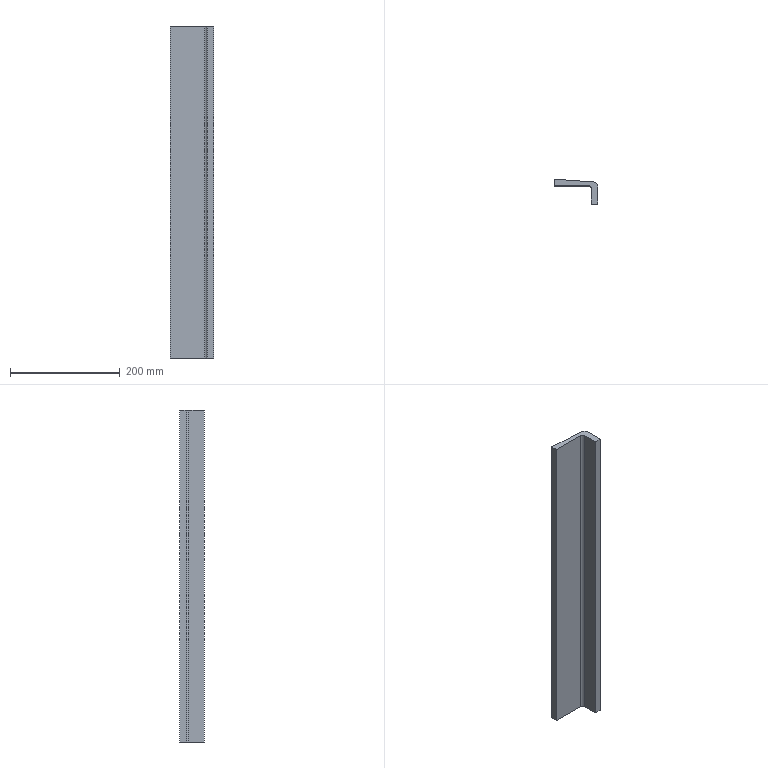Part | STEP file | daozhiban | 1 solid | 10 faces | box 80 x 45.5 x 606 mm | volume 689617 mm3 | plane 8 | cylinder 2 | commonest cylinder face diameters 10 x1 20 x1
STEP:
#1=CARTESIAN_POINT('',(0.,0.,0.));
#2=DIRECTION('',(0.,0.,1.));
#3=DIRECTION('',(1.,0.,0.));
#4=AXIS2_PLACEMENT_3D('',#1,#2,#3);
#5=CARTESIAN_POINT('',(36.453,-0.6319,-303.));
#6=VERTEX_POINT('',#5);
#7=CARTESIAN_POINT('',(29.053,9.024,-303.));
#8=VERTEX_POINT('',#7);
#9=CARTESIAN_POINT('',(26.453,-0.6319,-303.));
#10=DIRECTION('',(0.,0.,1.));
#11=DIRECTION('',(-1.,0.,0.));
#12=AXIS2_PLACEMENT_3D('',#9,#10,#11);
#13=CIRCLE('',#12,10.);
#14=CARTESIAN_POINT('',(26.453,-0.6319,303.));
#15=DIRECTION('',(0.,0.,-1.));
#16=DIRECTION('',(-1.,0.,0.));
#17=AXIS2_PLACEMENT_3D('',#14,#15,#16);
#18=CYLINDRICAL_SURFACE('',#17,10.);
#19=CARTESIAN_POINT('',(6.283,606.));
#20=DIRECTION('',(-1.,0.));
#21=VECTOR('',#20,1.);
#22=LINE('',#19,#21);
#23=(GEOMETRIC_REPRESENTATION_CONTEXT(2)PARAMETRIC_REPRESENTATION_CONTEXT()REPRESENTATION_CONTEXT('',''));
#24=DEFINITIONAL_REPRESENTATION('',(#22),#23);
#25=PCURVE('',#18,#24);
#26=CARTESIAN_POINT('',(26.453,-0.6319,-303.));
#27=DIRECTION('',(0.,0.,-1.));
#28=DIRECTION('',(-1.,0.,0.));
#29=AXIS2_PLACEMENT_3D('',#26,#27,#28);
#30=PLANE('',#29);
#31=CARTESIAN_POINT('',(10.,0.));
#32=CARTESIAN_POINT('',(10.,-17.321));
#33=CARTESIAN_POINT('',(-5.,-8.66));
#34=CARTESIAN_POINT('',(-20.,0.));
#35=CARTESIAN_POINT('',(-5.,8.66));
#36=CARTESIAN_POINT('',(10.,17.321));
#37=CARTESIAN_POINT('',(10.,0.));
#38=(BOUNDED_CURVE()B_SPLINE_CURVE(2,(#31,#32,#33,#34,#35,#36,#37),.UNSPECIFIED.,.T.,.F.)B_SPLINE_CURVE_WITH_KNOTS((1,2,2,2,2,1),(-2.094,0.,2.094,4.189,6.283,8.378),.UNSPECIFIED.)CURVE()GEOMETRIC_REPRESENTATION_ITEM()RATIONAL_B_SPLINE_CURVE((1.,0.5,1.,0.5,1.,0.5,1.))REPRESENTATION_ITEM(''));
#39=(GEOMETRIC_REPRESENTATION_CONTEXT(2)PARAMETRIC_REPRESENTATION_CONTEXT()REPRESENTATION_CONTEXT('',''));
#40=DEFINITIONAL_REPRESENTATION('',(#38),#39);
#41=PCURVE('',#30,#40);
#42=SURFACE_CURVE('',#13,(#25,#41),.PCURVE_S1.);
#43=EDGE_CURVE('',#6,#8,#42,.T.);
#44=ORIENTED_EDGE('',*,*,#43,.T.);
#45=CARTESIAN_POINT('',(29.053,9.024,303.));
#46=VERTEX_POINT('',#45);
#47=CARTESIAN_POINT('',(29.053,9.024,303.));
#48=DIRECTION('',(0.,0.,-1.));
#49=VECTOR('',#48,1.);
#50=LINE('',#47,#49);
#51=CARTESIAN_POINT('',(1.834,0.));
#52=DIRECTION('',(0.,1.));
#53=VECTOR('',#52,1.);
#54=LINE('',#51,#53);
#55=(GEOMETRIC_REPRESENTATION_CONTEXT(2)PARAMETRIC_REPRESENTATION_CONTEXT()REPRESENTATION_CONTEXT('',''));
#56=DEFINITIONAL_REPRESENTATION('',(#54),#55);
#57=PCURVE('',#18,#56);
#58=CARTESIAN_POINT('',(-43.547,13.847,303.));
#59=DIRECTION('',(-0.06629,-0.9978,0.));
#60=DIRECTION('',(0.9978,-0.06629,0.));
#61=AXIS2_PLACEMENT_3D('',#58,#59,#60);
#62=PLANE('',#61);
#63=CARTESIAN_POINT('',(72.76,0.));
#64=DIRECTION('',(0.,-1.));
#65=VECTOR('',#64,1.);
#66=LINE('',#63,#65);
#67=(GEOMETRIC_REPRESENTATION_CONTEXT(2)PARAMETRIC_REPRESENTATION_CONTEXT()REPRESENTATION_CONTEXT('',''));
#68=DEFINITIONAL_REPRESENTATION('',(#66),#67);
#69=PCURVE('',#62,#68);
#70=SURFACE_CURVE('',#50,(#57,#69),.PCURVE_S1.);
#71=EDGE_CURVE('',#46,#8,#70,.T.);
#72=ORIENTED_EDGE('',*,*,#71,.F.);
#73=CARTESIAN_POINT('',(36.453,-0.6319,303.));
#74=VERTEX_POINT('',#73);
#75=CARTESIAN_POINT('',(26.453,-0.6319,303.));
#76=DIRECTION('',(0.,0.,1.));
#77=DIRECTION('',(-1.,0.,0.));
#78=AXIS2_PLACEMENT_3D('',#75,#76,#77);
#79=CIRCLE('',#78,10.);
#80=CARTESIAN_POINT('',(6.283,0.));
#81=DIRECTION('',(-1.,0.));
#82=VECTOR('',#81,1.);
#83=LINE('',#80,#82);
#84=(GEOMETRIC_REPRESENTATION_CONTEXT(2)PARAMETRIC_REPRESENTATION_CONTEXT()REPRESENTATION_CONTEXT('',''));
#85=DEFINITIONAL_REPRESENTATION('',(#83),#84);
#86=PCURVE('',#18,#85);
#87=CARTESIAN_POINT('',(26.453,-0.6319,303.));
#88=DIRECTION('',(0.,0.,-1.));
#89=DIRECTION('',(-1.,0.,0.));
#90=AXIS2_PLACEMENT_3D('',#87,#88,#89);
#91=PLANE('',#90);
#92=CARTESIAN_POINT('',(10.,0.));
#93=CARTESIAN_POINT('',(10.,-17.321));
#94=CARTESIAN_POINT('',(-5.,-8.66));
#95=CARTESIAN_POINT('',(-20.,0.));
#96=CARTESIAN_POINT('',(-5.,8.66));
#97=CARTESIAN_POINT('',(10.,17.321));
#98=CARTESIAN_POINT('',(10.,0.));
#99=(BOUNDED_CURVE()B_SPLINE_CURVE(2,(#92,#93,#94,#95,#96,#97,#98),.UNSPECIFIED.,.T.,.F.)B_SPLINE_CURVE_WITH_KNOTS((1,2,2,2,2,1),(-2.094,0.,2.094,4.189,6.283,8.378),.UNSPECIFIED.)CURVE()GEOMETRIC_REPRESENTATION_ITEM()RATIONAL_B_SPLINE_CURVE((1.,0.5,1.,0.5,1.,0.5,1.))REPRESENTATION_ITEM(''));
#100=(GEOMETRIC_REPRESENTATION_CONTEXT(2)PARAMETRIC_REPRESENTATION_CONTEXT()REPRESENTATION_CONTEXT('',''));
#101=DEFINITIONAL_REPRESENTATION('',(#99),#100);
#102=PCURVE('',#91,#101);
#103=SURFACE_CURVE('',#79,(#86,#102),.PCURVE_S1.);
#104=EDGE_CURVE('',#74,#46,#103,.T.);
#105=ORIENTED_EDGE('',*,*,#104,.F.);
#106=CARTESIAN_POINT('',(36.453,-0.6319,303.));
#107=DIRECTION('',(0.,0.,-1.));
#108=VECTOR('',#107,1.);
#109=LINE('',#106,#108);
#110=CARTESIAN_POINT('',(3.142,0.));
#111=DIRECTION('',(0.,1.));
#112=VECTOR('',#111,1.);
#113=LINE('',#110,#112);
#114=(GEOMETRIC_REPRESENTATION_CONTEXT(2)PARAMETRIC_REPRESENTATION_CONTEXT()REPRESENTATION_CONTEXT('',''));
#115=DEFINITIONAL_REPRESENTATION('',(#113),#114);
#116=PCURVE('',#18,#115);
#117=CARTESIAN_POINT('',(36.453,-0.6319,303.));
#118=DIRECTION('',(-1.,0.,0.));
#119=DIRECTION('',(0.,-1.,0.));
#120=AXIS2_PLACEMENT_3D('',#117,#118,#119);
#121=PLANE('',#120);
#122=CARTESIAN_POINT('',(0.,0.));
#123=DIRECTION('',(0.,-1.));
#124=VECTOR('',#123,1.);
#125=LINE('',#122,#124);
#126=(GEOMETRIC_REPRESENTATION_CONTEXT(2)PARAMETRIC_REPRESENTATION_CONTEXT()REPRESENTATION_CONTEXT('',''));
#127=DEFINITIONAL_REPRESENTATION('',(#125),#126);
#128=PCURVE('',#121,#127);
#129=SURFACE_CURVE('',#109,(#116,#128),.PCURVE_S1.);
#130=EDGE_CURVE('',#74,#6,#129,.T.);
#131=ORIENTED_EDGE('',*,*,#130,.T.);
#132=EDGE_LOOP('',(#44,#72,#105,#131));
#133=FACE_BOUND('',#132,.T.);
#134=ADVANCED_FACE('',(#133),#18,.T.);
#135=CARTESIAN_POINT('',(-43.547,13.847,-303.));
#136=VERTEX_POINT('',#135);
#137=CARTESIAN_POINT('',(-43.547,13.847,-303.));
#138=DIRECTION('',(-0.9978,0.06629,0.));
#139=VECTOR('',#138,1.);
#140=LINE('',#137,#139);
#141=CARTESIAN_POINT('',(0.,-606.));
#142=DIRECTION('',(-1.,0.));
#143=VECTOR('',#142,1.);
#144=LINE('',#141,#143);
#145=(GEOMETRIC_REPRESENTATION_CONTEXT(2)PARAMETRIC_REPRESENTATION_CONTEXT()REPRESENTATION_CONTEXT('',''));
#146=DEFINITIONAL_REPRESENTATION('',(#144),#145);
#147=PCURVE('',#62,#146);
#148=CARTESIAN_POINT('',(70.,14.479));
#149=DIRECTION('',(0.9978,0.06629));
#150=VECTOR('',#149,1.);
#151=LINE('',#148,#150);
#152=(GEOMETRIC_REPRESENTATION_CONTEXT(2)PARAMETRIC_REPRESENTATION_CONTEXT()REPRESENTATION_CONTEXT('',''));
#153=DEFINITIONAL_REPRESENTATION('',(#151),#152);
#154=PCURVE('',#30,#153);
#155=SURFACE_CURVE('',#140,(#147,#154),.PCURVE_S1.);
#156=EDGE_CURVE('',#8,#136,#155,.T.);
#157=ORIENTED_EDGE('',*,*,#156,.T.);
#158=CARTESIAN_POINT('',(-43.547,13.847,303.));
#159=VERTEX_POINT('',#158);
#160=CARTESIAN_POINT('',(-43.547,13.847,303.));
#161=DIRECTION('',(0.,0.,-1.));
#162=VECTOR('',#161,1.);
#163=LINE('',#160,#162);
#164=CARTESIAN_POINT('',(0.,0.));
#165=DIRECTION('',(0.,-1.));
#166=VECTOR('',#165,1.);
#167=LINE('',#164,#166);
#168=(GEOMETRIC_REPRESENTATION_CONTEXT(2)PARAMETRIC_REPRESENTATION_CONTEXT()REPRESENTATION_CONTEXT('',''));
#169=DEFINITIONAL_REPRESENTATION('',(#167),#168);
#170=PCURVE('',#62,#169);
#171=CARTESIAN_POINT('',(-43.547,13.847,303.));
#172=DIRECTION('',(1.,0.,0.));
#173=DIRECTION('',(0.,0.,-1.));
#174=AXIS2_PLACEMENT_3D('',#171,#172,#173);
#175=PLANE('',#174);
#176=CARTESIAN_POINT('',(0.,0.));
#177=DIRECTION('',(1.,0.));
#178=VECTOR('',#177,1.);
#179=LINE('',#176,#178);
#180=(GEOMETRIC_REPRESENTATION_CONTEXT(2)PARAMETRIC_REPRESENTATION_CONTEXT()REPRESENTATION_CONTEXT('',''));
#181=DEFINITIONAL_REPRESENTATION('',(#179),#180);
#182=PCURVE('',#175,#181);
#183=SURFACE_CURVE('',#163,(#170,#182),.PCURVE_S1.);
#184=EDGE_CURVE('',#159,#136,#183,.T.);
#185=ORIENTED_EDGE('',*,*,#184,.F.);
#186=CARTESIAN_POINT('',(-43.547,13.847,303.));
#187=DIRECTION('',(-0.9978,0.06629,0.));
#188=VECTOR('',#187,1.);
#189=LINE('',#186,#188);
#190=CARTESIAN_POINT('',(0.,0.));
#191=DIRECTION('',(-1.,0.));
#192=VECTOR('',#191,1.);
#193=LINE('',#190,#192);
#194=(GEOMETRIC_REPRESENTATION_CONTEXT(2)PARAMETRIC_REPRESENTATION_CONTEXT()REPRESENTATION_CONTEXT('',''));
#195=DEFINITIONAL_REPRESENTATION('',(#193),#194);
#196=PCURVE('',#62,#195);
#197=CARTESIAN_POINT('',(70.,14.479));
#198=DIRECTION('',(0.9978,0.06629));
#199=VECTOR('',#198,1.);
#200=LINE('',#197,#199);
#201=(GEOMETRIC_REPRESENTATION_CONTEXT(2)PARAMETRIC_REPRESENTATION_CONTEXT()REPRESENTATION_CONTEXT('',''));
#202=DEFINITIONAL_REPRESENTATION('',(#200),#201);
#203=PCURVE('',#91,#202);
#204=SURFACE_CURVE('',#189,(#196,#203),.PCURVE_S1.);
#205=EDGE_CURVE('',#46,#159,#204,.T.);
#206=ORIENTED_EDGE('',*,*,#205,.F.);
#207=ORIENTED_EDGE('',*,*,#71,.T.);
#208=EDGE_LOOP('',(#157,#185,#206,#207));
#209=FACE_BOUND('',#208,.T.);
#210=ADVANCED_FACE('',(#209),#62,.F.);
#211=CARTESIAN_POINT('',(-43.547,1.847,-303.));
#212=VERTEX_POINT('',#211);
#213=CARTESIAN_POINT('',(-43.547,13.847,-303.));
#214=DIRECTION('',(0.,-1.,0.));
#215=VECTOR('',#214,1.);
#216=LINE('',#213,#215);
#217=CARTESIAN_POINT('',(606.,0.));
#218=DIRECTION('',(0.,-1.));
#219=VECTOR('',#218,1.);
#220=LINE('',#217,#219);
#221=(GEOMETRIC_REPRESENTATION_CONTEXT(2)PARAMETRIC_REPRESENTATION_CONTEXT()REPRESENTATION_CONTEXT('',''));
#222=DEFINITIONAL_REPRESENTATION('',(#220),#221);
#223=PCURVE('',#175,#222);
#224=CARTESIAN_POINT('',(70.,14.479));
#225=DIRECTION('',(0.,-1.));
#226=VECTOR('',#225,1.);
#227=LINE('',#224,#226);
#228=(GEOMETRIC_REPRESENTATION_CONTEXT(2)PARAMETRIC_REPRESENTATION_CONTEXT()REPRESENTATION_CONTEXT('',''));
#229=DEFINITIONAL_REPRESENTATION('',(#227),#228);
#230=PCURVE('',#30,#229);
#231=SURFACE_CURVE('',#216,(#223,#230),.PCURVE_S1.);
#232=EDGE_CURVE('',#136,#212,#231,.T.);
#233=ORIENTED_EDGE('',*,*,#232,.T.);
#234=CARTESIAN_POINT('',(-43.547,1.847,303.));
#235=VERTEX_POINT('',#234);
#236=CARTESIAN_POINT('',(-43.547,1.847,303.));
#237=DIRECTION('',(0.,0.,-1.));
#238=VECTOR('',#237,1.);
#239=LINE('',#236,#238);
#240=CARTESIAN_POINT('',(0.,-12.));
#241=DIRECTION('',(1.,0.));
#242=VECTOR('',#241,1.);
#243=LINE('',#240,#242);
#244=(GEOMETRIC_REPRESENTATION_CONTEXT(2)PARAMETRIC_REPRESENTATION_CONTEXT()REPRESENTATION_CONTEXT('',''));
#245=DEFINITIONAL_REPRESENTATION('',(#243),#244);
#246=PCURVE('',#175,#245);
#247=CARTESIAN_POINT('',(-43.547,1.847,303.));
#248=DIRECTION('',(0.,1.,0.));
#249=DIRECTION('',(0.,0.,1.));
#250=AXIS2_PLACEMENT_3D('',#247,#248,#249);
#251=PLANE('',#250);
#252=CARTESIAN_POINT('',(0.,0.));
#253=DIRECTION('',(-1.,0.));
#254=VECTOR('',#253,1.);
#255=LINE('',#252,#254);
#256=(GEOMETRIC_REPRESENTATION_CONTEXT(2)PARAMETRIC_REPRESENTATION_CONTEXT()REPRESENTATION_CONTEXT('',''));
#257=DEFINITIONAL_REPRESENTATION('',(#255),#256);
#258=PCURVE('',#251,#257);
#259=SURFACE_CURVE('',#239,(#246,#258),.PCURVE_S1.);
#260=EDGE_CURVE('',#235,#212,#259,.T.);
#261=ORIENTED_EDGE('',*,*,#260,.F.);
#262=CARTESIAN_POINT('',(-43.547,13.847,303.));
#263=DIRECTION('',(0.,-1.,0.));
#264=VECTOR('',#263,1.);
#265=LINE('',#262,#264);
#266=CARTESIAN_POINT('',(0.,0.));
#267=DIRECTION('',(0.,-1.));
#268=VECTOR('',#267,1.);
#269=LINE('',#266,#268);
#270=(GEOMETRIC_REPRESENTATION_CONTEXT(2)PARAMETRIC_REPRESENTATION_CONTEXT()REPRESENTATION_CONTEXT('',''));
#271=DEFINITIONAL_REPRESENTATION('',(#269),#270);
#272=PCURVE('',#175,#271);
#273=CARTESIAN_POINT('',(70.,14.479));
#274=DIRECTION('',(0.,-1.));
#275=VECTOR('',#274,1.);
#276=LINE('',#273,#275);
#277=(GEOMETRIC_REPRESENTATION_CONTEXT(2)PARAMETRIC_REPRESENTATION_CONTEXT()REPRESENTATION_CONTEXT('',''));
#278=DEFINITIONAL_REPRESENTATION('',(#276),#277);
#279=PCURVE('',#91,#278);
#280=SURFACE_CURVE('',#265,(#272,#279),.PCURVE_S1.);
#281=EDGE_CURVE('',#159,#235,#280,.T.);
#282=ORIENTED_EDGE('',*,*,#281,.F.);
#283=ORIENTED_EDGE('',*,*,#184,.T.);
#284=EDGE_LOOP('',(#233,#261,#282,#283));
#285=FACE_BOUND('',#284,.T.);
#286=ADVANCED_FACE('',(#285),#175,.F.);
#287=CARTESIAN_POINT('',(19.453,1.847,-303.));
#288=VERTEX_POINT('',#287);
#289=CARTESIAN_POINT('',(-43.547,1.847,-303.));
#290=DIRECTION('',(1.,0.,0.));
#291=VECTOR('',#290,1.);
#292=LINE('',#289,#291);
#293=CARTESIAN_POINT('',(-606.,0.));
#294=DIRECTION('',(0.,1.));
#295=VECTOR('',#294,1.);
#296=LINE('',#293,#295);
#297=(GEOMETRIC_REPRESENTATION_CONTEXT(2)PARAMETRIC_REPRESENTATION_CONTEXT()REPRESENTATION_CONTEXT('',''));
#298=DEFINITIONAL_REPRESENTATION('',(#296),#297);
#299=PCURVE('',#251,#298);
#300=CARTESIAN_POINT('',(70.,2.479));
#301=DIRECTION('',(-1.,0.));
#302=VECTOR('',#301,1.);
#303=LINE('',#300,#302);
#304=(GEOMETRIC_REPRESENTATION_CONTEXT(2)PARAMETRIC_REPRESENTATION_CONTEXT()REPRESENTATION_CONTEXT('',''));
#305=DEFINITIONAL_REPRESENTATION('',(#303),#304);
#306=PCURVE('',#30,#305);
#307=SURFACE_CURVE('',#292,(#299,#306),.PCURVE_S1.);
#308=EDGE_CURVE('',#212,#288,#307,.T.);
#309=ORIENTED_EDGE('',*,*,#308,.T.);
#310=CARTESIAN_POINT('',(19.453,1.847,303.));
#311=VERTEX_POINT('',#310);
#312=CARTESIAN_POINT('',(19.453,1.847,303.));
#313=DIRECTION('',(0.,0.,1.));
#314=VECTOR('',#313,1.);
#315=LINE('',#312,#314);
#316=CARTESIAN_POINT('',(0.,63.));
#317=DIRECTION('',(1.,0.));
#318=VECTOR('',#317,1.);
#319=LINE('',#316,#318);
#320=(GEOMETRIC_REPRESENTATION_CONTEXT(2)PARAMETRIC_REPRESENTATION_CONTEXT()REPRESENTATION_CONTEXT('',''));
#321=DEFINITIONAL_REPRESENTATION('',(#319),#320);
#322=PCURVE('',#251,#321);
#323=CARTESIAN_POINT('',(19.453,-3.153,303.));
#324=DIRECTION('',(0.,0.,1.));
#325=DIRECTION('',(1.,0.,0.));
#326=AXIS2_PLACEMENT_3D('',#323,#324,#325);
#327=CYLINDRICAL_SURFACE('',#326,5.);
#328=CARTESIAN_POINT('',(1.571,0.));
#329=DIRECTION('',(0.,1.));
#330=VECTOR('',#329,1.);
#331=LINE('',#328,#330);
#332=(GEOMETRIC_REPRESENTATION_CONTEXT(2)PARAMETRIC_REPRESENTATION_CONTEXT()REPRESENTATION_CONTEXT('',''));
#333=DEFINITIONAL_REPRESENTATION('',(#331),#332);
#334=PCURVE('',#327,#333);
#335=SURFACE_CURVE('',#315,(#322,#334),.PCURVE_S1.);
#336=EDGE_CURVE('',#288,#311,#335,.T.);
#337=ORIENTED_EDGE('',*,*,#336,.T.);
#338=CARTESIAN_POINT('',(-43.547,1.847,303.));
#339=DIRECTION('',(1.,0.,0.));
#340=VECTOR('',#339,1.);
#341=LINE('',#338,#340);
#342=CARTESIAN_POINT('',(0.,0.));
#343=DIRECTION('',(0.,1.));
#344=VECTOR('',#343,1.);
#345=LINE('',#342,#344);
#346=(GEOMETRIC_REPRESENTATION_CONTEXT(2)PARAMETRIC_REPRESENTATION_CONTEXT()REPRESENTATION_CONTEXT('',''));
#347=DEFINITIONAL_REPRESENTATION('',(#345),#346);
#348=PCURVE('',#251,#347);
#349=CARTESIAN_POINT('',(70.,2.479));
#350=DIRECTION('',(-1.,0.));
#351=VECTOR('',#350,1.);
#352=LINE('',#349,#351);
#353=(GEOMETRIC_REPRESENTATION_CONTEXT(2)PARAMETRIC_REPRESENTATION_CONTEXT()REPRESENTATION_CONTEXT('',''));
#354=DEFINITIONAL_REPRESENTATION('',(#352),#353);
#355=PCURVE('',#91,#354);
#356=SURFACE_CURVE('',#341,(#348,#355),.PCURVE_S1.);
#357=EDGE_CURVE('',#235,#311,#356,.T.);
#358=ORIENTED_EDGE('',*,*,#357,.F.);
#359=ORIENTED_EDGE('',*,*,#260,.T.);
#360=EDGE_LOOP('',(#309,#337,#358,#359));
#361=FACE_BOUND('',#360,.T.);
#362=ADVANCED_FACE('',(#361),#251,.F.);
#363=CARTESIAN_POINT('',(24.453,-3.153,303.));
#364=VERTEX_POINT('',#363);
#365=CARTESIAN_POINT('',(24.453,-31.653,303.));
#366=VERTEX_POINT('',#365);
#367=CARTESIAN_POINT('',(24.453,1.847,303.));
#368=DIRECTION('',(0.,-1.,0.));
#369=VECTOR('',#368,1.);
#370=LINE('',#367,#369);
#371=CARTESIAN_POINT('',(24.453,1.847,303.));
#372=DIRECTION('',(1.,0.,0.));
#373=DIRECTION('',(0.,1.,0.));
#374=AXIS2_PLACEMENT_3D('',#371,#372,#373);
#375=PLANE('',#374);
#376=CARTESIAN_POINT('',(0.,0.));
#377=DIRECTION('',(-1.,0.));
#378=VECTOR('',#377,1.);
#379=LINE('',#376,#378);
#380=(GEOMETRIC_REPRESENTATION_CONTEXT(2)PARAMETRIC_REPRESENTATION_CONTEXT()REPRESENTATION_CONTEXT('',''));
#381=DEFINITIONAL_REPRESENTATION('',(#379),#380);
#382=PCURVE('',#375,#381);
#383=CARTESIAN_POINT('',(2.,2.479));
#384=DIRECTION('',(0.,-1.));
#385=VECTOR('',#384,1.);
#386=LINE('',#383,#385);
#387=(GEOMETRIC_REPRESENTATION_CONTEXT(2)PARAMETRIC_REPRESENTATION_CONTEXT()REPRESENTATION_CONTEXT('',''));
#388=DEFINITIONAL_REPRESENTATION('',(#386),#387);
#389=PCURVE('',#91,#388);
#390=SURFACE_CURVE('',#370,(#382,#389),.PCURVE_S1.);
#391=EDGE_CURVE('',#364,#366,#390,.T.);
#392=ORIENTED_EDGE('',*,*,#391,.F.);
#393=CARTESIAN_POINT('',(24.453,-3.153,-303.));
#394=VERTEX_POINT('',#393);
#395=CARTESIAN_POINT('',(24.453,-3.153,-303.));
#396=DIRECTION('',(0.,0.,-1.));
#397=VECTOR('',#396,1.);
#398=LINE('',#395,#397);
#399=CARTESIAN_POINT('',(-5.,-606.));
#400=DIRECTION('',(0.,-1.));
#401=VECTOR('',#400,1.);
#402=LINE('',#399,#401);
#403=(GEOMETRIC_REPRESENTATION_CONTEXT(2)PARAMETRIC_REPRESENTATION_CONTEXT()REPRESENTATION_CONTEXT('',''));
#404=DEFINITIONAL_REPRESENTATION('',(#402),#403);
#405=PCURVE('',#375,#404);
#406=CARTESIAN_POINT('',(0.,-606.));
#407=DIRECTION('',(0.,-1.));
#408=VECTOR('',#407,1.);
#409=LINE('',#406,#408);
#410=(GEOMETRIC_REPRESENTATION_CONTEXT(2)PARAMETRIC_REPRESENTATION_CONTEXT()REPRESENTATION_CONTEXT('',''));
#411=DEFINITIONAL_REPRESENTATION('',(#409),#410);
#412=PCURVE('',#327,#411);
#413=SURFACE_CURVE('',#398,(#405,#412),.PCURVE_S1.);
#414=EDGE_CURVE('',#364,#394,#413,.T.);
#415=ORIENTED_EDGE('',*,*,#414,.T.);
#416=CARTESIAN_POINT('',(24.453,-31.653,-303.));
#417=VERTEX_POINT('',#416);
#418=CARTESIAN_POINT('',(24.453,1.847,-303.));
#419=DIRECTION('',(0.,-1.,0.));
#420=VECTOR('',#419,1.);
#421=LINE('',#418,#420);
#422=CARTESIAN_POINT('',(0.,-606.));
#423=DIRECTION('',(-1.,0.));
#424=VECTOR('',#423,1.);
#425=LINE('',#422,#424);
#426=(GEOMETRIC_REPRESENTATION_CONTEXT(2)PARAMETRIC_REPRESENTATION_CONTEXT()REPRESENTATION_CONTEXT('',''));
#427=DEFINITIONAL_REPRESENTATION('',(#425),#426);
#428=PCURVE('',#375,#427);
#429=CARTESIAN_POINT('',(2.,2.479));
#430=DIRECTION('',(0.,-1.));
#431=VECTOR('',#430,1.);
#432=LINE('',#429,#431);
#433=(GEOMETRIC_REPRESENTATION_CONTEXT(2)PARAMETRIC_REPRESENTATION_CONTEXT()REPRESENTATION_CONTEXT('',''));
#434=DEFINITIONAL_REPRESENTATION('',(#432),#433);
#435=PCURVE('',#30,#434);
#436=SURFACE_CURVE('',#421,(#428,#435),.PCURVE_S1.);
#437=EDGE_CURVE('',#394,#417,#436,.T.);
#438=ORIENTED_EDGE('',*,*,#437,.T.);
#439=CARTESIAN_POINT('',(24.453,-31.653,303.));
#440=DIRECTION('',(0.,0.,-1.));
#441=VECTOR('',#440,1.);
#442=LINE('',#439,#441);
#443=CARTESIAN_POINT('',(-33.5,0.));
#444=DIRECTION('',(0.,-1.));
#445=VECTOR('',#444,1.);
#446=LINE('',#443,#445);
#447=(GEOMETRIC_REPRESENTATION_CONTEXT(2)PARAMETRIC_REPRESENTATION_CONTEXT()REPRESENTATION_CONTEXT('',''));
#448=DEFINITIONAL_REPRESENTATION('',(#446),#447);
#449=PCURVE('',#375,#448);
#450=CARTESIAN_POINT('',(24.453,-31.653,303.));
#451=DIRECTION('',(0.,1.,0.));
#452=DIRECTION('',(0.,0.,1.));
#453=AXIS2_PLACEMENT_3D('',#450,#451,#452);
#454=PLANE('',#453);
#455=CARTESIAN_POINT('',(0.,0.));
#456=DIRECTION('',(-1.,0.));
#457=VECTOR('',#456,1.);
#458=LINE('',#455,#457);
#459=(GEOMETRIC_REPRESENTATION_CONTEXT(2)PARAMETRIC_REPRESENTATION_CONTEXT()REPRESENTATION_CONTEXT('',''));
#460=DEFINITIONAL_REPRESENTATION('',(#458),#459);
#461=PCURVE('',#454,#460);
#462=SURFACE_CURVE('',#442,(#449,#461),.PCURVE_S1.);
#463=EDGE_CURVE('',#366,#417,#462,.T.);
#464=ORIENTED_EDGE('',*,*,#463,.F.);
#465=EDGE_LOOP('',(#392,#415,#438,#464));
#466=FACE_BOUND('',#465,.T.);
#467=ADVANCED_FACE('',(#466),#375,.F.);
#468=CARTESIAN_POINT('',(36.453,-31.653,-303.));
#469=VERTEX_POINT('',#468);
#470=CARTESIAN_POINT('',(24.453,-31.653,-303.));
#471=DIRECTION('',(1.,0.,0.));
#472=VECTOR('',#471,1.);
#473=LINE('',#470,#472);
#474=CARTESIAN_POINT('',(-606.,0.));
#475=DIRECTION('',(0.,1.));
#476=VECTOR('',#475,1.);
#477=LINE('',#474,#476);
#478=(GEOMETRIC_REPRESENTATION_CONTEXT(2)PARAMETRIC_REPRESENTATION_CONTEXT()REPRESENTATION_CONTEXT('',''));
#479=DEFINITIONAL_REPRESENTATION('',(#477),#478);
#480=PCURVE('',#454,#479);
#481=CARTESIAN_POINT('',(2.,-31.021));
#482=DIRECTION('',(-1.,0.));
#483=VECTOR('',#482,1.);
#484=LINE('',#481,#483);
#485=(GEOMETRIC_REPRESENTATION_CONTEXT(2)PARAMETRIC_REPRESENTATION_CONTEXT()REPRESENTATION_CONTEXT('',''));
#486=DEFINITIONAL_REPRESENTATION('',(#484),#485);
#487=PCURVE('',#30,#486);
#488=SURFACE_CURVE('',#473,(#480,#487),.PCURVE_S1.);
#489=EDGE_CURVE('',#417,#469,#488,.T.);
#490=ORIENTED_EDGE('',*,*,#489,.T.);
#491=CARTESIAN_POINT('',(36.453,-31.653,303.));
#492=VERTEX_POINT('',#491);
#493=CARTESIAN_POINT('',(36.453,-31.653,303.));
#494=DIRECTION('',(0.,0.,-1.));
#495=VECTOR('',#494,1.);
#496=LINE('',#493,#495);
#497=CARTESIAN_POINT('',(0.,12.));
#498=DIRECTION('',(-1.,0.));
#499=VECTOR('',#498,1.);
#500=LINE('',#497,#499);
#501=(GEOMETRIC_REPRESENTATION_CONTEXT(2)PARAMETRIC_REPRESENTATION_CONTEXT()REPRESENTATION_CONTEXT('',''));
#502=DEFINITIONAL_REPRESENTATION('',(#500),#501);
#503=PCURVE('',#454,#502);
#504=CARTESIAN_POINT('',(31.021,0.));
#505=DIRECTION('',(0.,-1.));
#506=VECTOR('',#505,1.);
#507=LINE('',#504,#506);
#508=(GEOMETRIC_REPRESENTATION_CONTEXT(2)PARAMETRIC_REPRESENTATION_CONTEXT()REPRESENTATION_CONTEXT('',''));
#509=DEFINITIONAL_REPRESENTATION('',(#507),#508);
#510=PCURVE('',#121,#509);
#511=SURFACE_CURVE('',#496,(#503,#510),.PCURVE_S1.);
#512=EDGE_CURVE('',#492,#469,#511,.T.);
#513=ORIENTED_EDGE('',*,*,#512,.F.);
#514=CARTESIAN_POINT('',(24.453,-31.653,303.));
#515=DIRECTION('',(1.,0.,0.));
#516=VECTOR('',#515,1.);
#517=LINE('',#514,#516);
#518=CARTESIAN_POINT('',(0.,0.));
#519=DIRECTION('',(0.,1.));
#520=VECTOR('',#519,1.);
#521=LINE('',#518,#520);
#522=(GEOMETRIC_REPRESENTATION_CONTEXT(2)PARAMETRIC_REPRESENTATION_CONTEXT()REPRESENTATION_CONTEXT('',''));
#523=DEFINITIONAL_REPRESENTATION('',(#521),#522);
#524=PCURVE('',#454,#523);
#525=CARTESIAN_POINT('',(2.,-31.021));
#526=DIRECTION('',(-1.,0.));
#527=VECTOR('',#526,1.);
#528=LINE('',#525,#527);
#529=(GEOMETRIC_REPRESENTATION_CONTEXT(2)PARAMETRIC_REPRESENTATION_CONTEXT()REPRESENTATION_CONTEXT('',''));
#530=DEFINITIONAL_REPRESENTATION('',(#528),#529);
#531=PCURVE('',#91,#530);
#532=SURFACE_CURVE('',#517,(#524,#531),.PCURVE_S1.);
#533=EDGE_CURVE('',#366,#492,#532,.T.);
#534=ORIENTED_EDGE('',*,*,#533,.F.);
#535=ORIENTED_EDGE('',*,*,#463,.T.);
#536=EDGE_LOOP('',(#490,#513,#534,#535));
#537=FACE_BOUND('',#536,.T.);
#538=ADVANCED_FACE('',(#537),#454,.F.);
#539=CARTESIAN_POINT('',(36.453,-0.6319,-303.));
#540=DIRECTION('',(0.,1.,0.));
#541=VECTOR('',#540,1.);
#542=LINE('',#539,#541);
#543=CARTESIAN_POINT('',(0.,-606.));
#544=DIRECTION('',(-1.,0.));
#545=VECTOR('',#544,1.);
#546=LINE('',#543,#545);
#547=(GEOMETRIC_REPRESENTATION_CONTEXT(2)PARAMETRIC_REPRESENTATION_CONTEXT()REPRESENTATION_CONTEXT('',''));
#548=DEFINITIONAL_REPRESENTATION('',(#546),#547);
#549=PCURVE('',#121,#548);
#550=CARTESIAN_POINT('',(-10.,0.));
#551=DIRECTION('',(0.,1.));
#552=VECTOR('',#551,1.);
#553=LINE('',#550,#552);
#554=(GEOMETRIC_REPRESENTATION_CONTEXT(2)PARAMETRIC_REPRESENTATION_CONTEXT()REPRESENTATION_CONTEXT('',''));
#555=DEFINITIONAL_REPRESENTATION('',(#553),#554);
#556=PCURVE('',#30,#555);
#557=SURFACE_CURVE('',#542,(#549,#556),.PCURVE_S1.);
#558=EDGE_CURVE('',#469,#6,#557,.T.);
#559=ORIENTED_EDGE('',*,*,#558,.T.);
#560=ORIENTED_EDGE('',*,*,#130,.F.);
#561=CARTESIAN_POINT('',(36.453,-0.6319,303.));
#562=DIRECTION('',(0.,1.,0.));
#563=VECTOR('',#562,1.);
#564=LINE('',#561,#563);
#565=CARTESIAN_POINT('',(0.,0.));
#566=DIRECTION('',(-1.,0.));
#567=VECTOR('',#566,1.);
#568=LINE('',#565,#567);
#569=(GEOMETRIC_REPRESENTATION_CONTEXT(2)PARAMETRIC_REPRESENTATION_CONTEXT()REPRESENTATION_CONTEXT('',''));
#570=DEFINITIONAL_REPRESENTATION('',(#568),#569);
#571=PCURVE('',#121,#570);
#572=CARTESIAN_POINT('',(-10.,0.));
#573=DIRECTION('',(0.,1.));
#574=VECTOR('',#573,1.);
#575=LINE('',#572,#574);
#576=(GEOMETRIC_REPRESENTATION_CONTEXT(2)PARAMETRIC_REPRESENTATION_CONTEXT()REPRESENTATION_CONTEXT('',''));
#577=DEFINITIONAL_REPRESENTATION('',(#575),#576);
#578=PCURVE('',#91,#577);
#579=SURFACE_CURVE('',#564,(#571,#578),.PCURVE_S1.);
#580=EDGE_CURVE('',#492,#74,#579,.T.);
#581=ORIENTED_EDGE('',*,*,#580,.F.);
#582=ORIENTED_EDGE('',*,*,#512,.T.);
#583=EDGE_LOOP('',(#559,#560,#581,#582));
#584=FACE_BOUND('',#583,.T.);
#585=ADVANCED_FACE('',(#584),#121,.F.);
#586=ORIENTED_EDGE('',*,*,#104,.T.);
#587=ORIENTED_EDGE('',*,*,#205,.T.);
#588=ORIENTED_EDGE('',*,*,#281,.T.);
#589=ORIENTED_EDGE('',*,*,#357,.T.);
#590=CARTESIAN_POINT('',(19.453,-3.153,303.));
#591=DIRECTION('',(0.,0.,-1.));
#592=DIRECTION('',(-1.,0.,0.));
#593=AXIS2_PLACEMENT_3D('',#590,#591,#592);
#594=CIRCLE('',#593,5.);
#595=CARTESIAN_POINT('',(7.,-2.521));
#596=DIRECTION('',(1.,0.));
#597=AXIS2_PLACEMENT_2D('',#595,#596);
#598=CIRCLE('',#597,5.);
#599=(GEOMETRIC_REPRESENTATION_CONTEXT(2)PARAMETRIC_REPRESENTATION_CONTEXT()REPRESENTATION_CONTEXT('',''));
#600=DEFINITIONAL_REPRESENTATION('',(#598),#599);
#601=PCURVE('',#91,#600);
#602=CARTESIAN_POINT('',(3.142,0.));
#603=DIRECTION('',(-1.,0.));
#604=VECTOR('',#603,1.);
#605=LINE('',#602,#604);
#606=(GEOMETRIC_REPRESENTATION_CONTEXT(2)PARAMETRIC_REPRESENTATION_CONTEXT()REPRESENTATION_CONTEXT('',''));
#607=DEFINITIONAL_REPRESENTATION('',(#605),#606);
#608=PCURVE('',#327,#607);
#609=SURFACE_CURVE('',#594,(#601,#608),.PCURVE_S1.);
#610=EDGE_CURVE('',#311,#364,#609,.T.);
#611=ORIENTED_EDGE('',*,*,#610,.T.);
#612=ORIENTED_EDGE('',*,*,#391,.T.);
#613=ORIENTED_EDGE('',*,*,#533,.T.);
#614=ORIENTED_EDGE('',*,*,#580,.T.);
#615=EDGE_LOOP('',(#586,#587,#588,#589,#611,#612,#613,#614));
#616=FACE_BOUND('',#615,.T.);
#617=ADVANCED_FACE('',(#616),#91,.F.);
#618=ORIENTED_EDGE('',*,*,#43,.F.);
#619=ORIENTED_EDGE('',*,*,#558,.F.);
#620=ORIENTED_EDGE('',*,*,#489,.F.);
#621=ORIENTED_EDGE('',*,*,#437,.F.);
#622=CARTESIAN_POINT('',(19.453,-3.153,-303.));
#623=DIRECTION('',(0.,0.,1.));
#624=DIRECTION('',(-1.,0.,0.));
#625=AXIS2_PLACEMENT_3D('',#622,#623,#624);
#626=CIRCLE('',#625,5.);
#627=CARTESIAN_POINT('',(12.,-2.521));
#628=CARTESIAN_POINT('',(12.,-11.181));
#629=CARTESIAN_POINT('',(4.5,-6.851));
#630=CARTESIAN_POINT('',(-3.,-2.521));
#631=CARTESIAN_POINT('',(4.5,1.809));
#632=CARTESIAN_POINT('',(12.,6.139));
#633=CARTESIAN_POINT('',(12.,-2.521));
#634=(BOUNDED_CURVE()B_SPLINE_CURVE(2,(#627,#628,#629,#630,#631,#632,#633),.UNSPECIFIED.,.T.,.F.)B_SPLINE_CURVE_WITH_KNOTS((1,2,2,2,2,1),(-2.094,0.,2.094,4.189,6.283,8.378),.UNSPECIFIED.)CURVE()GEOMETRIC_REPRESENTATION_ITEM()RATIONAL_B_SPLINE_CURVE((1.,0.5,1.,0.5,1.,0.5,1.))REPRESENTATION_ITEM(''));
#635=(GEOMETRIC_REPRESENTATION_CONTEXT(2)PARAMETRIC_REPRESENTATION_CONTEXT()REPRESENTATION_CONTEXT('',''));
#636=DEFINITIONAL_REPRESENTATION('',(#634),#635);
#637=PCURVE('',#30,#636);
#638=CARTESIAN_POINT('',(-3.142,-606.));
#639=DIRECTION('',(1.,0.));
#640=VECTOR('',#639,1.);
#641=LINE('',#638,#640);
#642=(GEOMETRIC_REPRESENTATION_CONTEXT(2)PARAMETRIC_REPRESENTATION_CONTEXT()REPRESENTATION_CONTEXT('',''));
#643=DEFINITIONAL_REPRESENTATION('',(#641),#642);
#644=PCURVE('',#327,#643);
#645=SURFACE_CURVE('',#626,(#637,#644),.PCURVE_S1.);
#646=EDGE_CURVE('',#394,#288,#645,.T.);
#647=ORIENTED_EDGE('',*,*,#646,.T.);
#648=ORIENTED_EDGE('',*,*,#308,.F.);
#649=ORIENTED_EDGE('',*,*,#232,.F.);
#650=ORIENTED_EDGE('',*,*,#156,.F.);
#651=EDGE_LOOP('',(#618,#619,#620,#621,#647,#648,#649,#650));
#652=FACE_BOUND('',#651,.T.);
#653=ADVANCED_FACE('',(#652),#30,.T.);
#654=ORIENTED_EDGE('',*,*,#414,.T.);
#655=ORIENTED_EDGE('',*,*,#646,.T.);
#656=ORIENTED_EDGE('',*,*,#336,.T.);
#657=ORIENTED_EDGE('',*,*,#610,.T.);
#658=EDGE_LOOP('',(#654,#655,#656,#657));
#659=FACE_BOUND('',#658,.F.);
#660=ADVANCED_FACE('',(#659),#327,.F.);
#661=CLOSED_SHELL('',(#134,#210,#286,#362,#467,#538,#585,#617,#653,#660));
#662=MANIFOLD_SOLID_BREP('',#661);
#663=(LENGTH_UNIT()NAMED_UNIT(*)SI_UNIT(.MILLI.,.METRE.));
#664=UNCERTAINTY_MEASURE_WITH_UNIT(LENGTH_MEASURE(0.0000001),#663,'','');
#665=(NAMED_UNIT(*)PLANE_ANGLE_UNIT()SI_UNIT($,.RADIAN.));
#666=(NAMED_UNIT(*)SI_UNIT($,.STERADIAN.)SOLID_ANGLE_UNIT());
#667=(GEOMETRIC_REPRESENTATION_CONTEXT(3)GLOBAL_UNCERTAINTY_ASSIGNED_CONTEXT((#664))GLOBAL_UNIT_ASSIGNED_CONTEXT((#663,#665,#666))REPRESENTATION_CONTEXT('',''));
#668=ADVANCED_BREP_SHAPE_REPRESENTATION('',(#4,#662),#667);